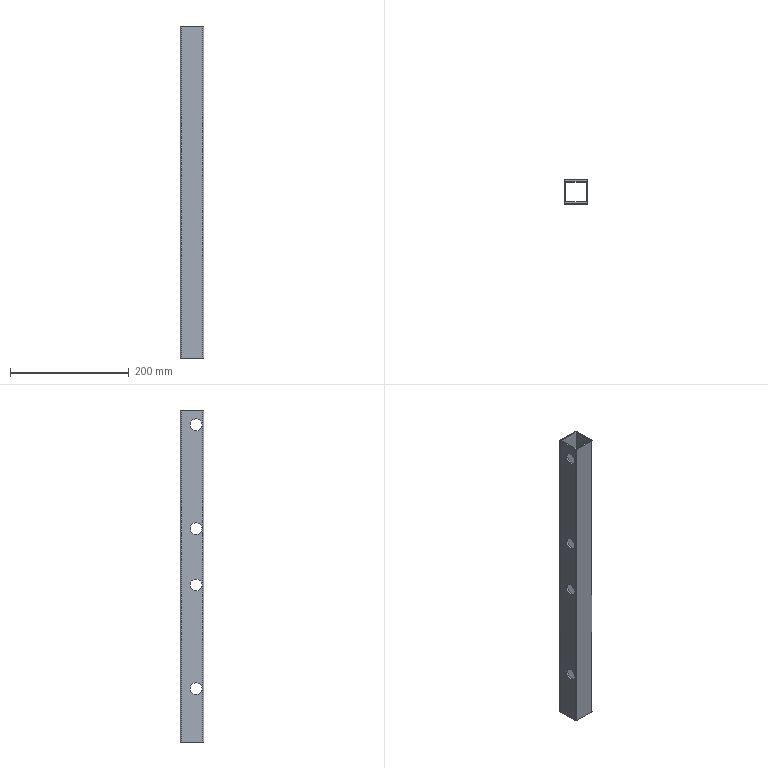Part | STEP file | X77-09107 | 1 solid | 30 faces | box 40 x 40 x 560 mm | volume 239177 mm3 | cylinder 20 | plane 10 | commonest cylinder face diameters 20 x16 4 x4
STEP:
#1=CARTESIAN_POINT('',(0.,3.,90.));
#2=VERTEX_POINT('',#1);
#3=CARTESIAN_POINT('',(0.,23.,90.));
#4=VERTEX_POINT('',#3);
#5=CARTESIAN_POINT('',(0.,13.,90.));
#6=DIRECTION('',(1.,0.,0.));
#7=DIRECTION('',(0.,1.,0.));
#8=AXIS2_PLACEMENT_3D('',#5,#6,#7);
#9=CIRCLE('',#8,10.);
#10=EDGE_CURVE('',#2,#4,#9,.T.);
#11=ORIENTED_EDGE('',*,*,#10,.F.);
#12=CARTESIAN_POINT('',(3.,3.,90.));
#13=VERTEX_POINT('',#12);
#14=CARTESIAN_POINT('',(0.,3.,90.));
#15=DIRECTION('',(1.,0.,0.));
#16=VECTOR('',#15,1000.);
#17=LINE('',#14,#16);
#18=EDGE_CURVE('',#2,#13,#17,.T.);
#19=ORIENTED_EDGE('',*,*,#18,.T.);
#20=CARTESIAN_POINT('',(3.,23.,90.));
#21=VERTEX_POINT('',#20);
#22=CARTESIAN_POINT('',(3.,13.,90.));
#23=DIRECTION('',(1.,0.,0.));
#24=DIRECTION('',(0.,0.,-1.));
#25=AXIS2_PLACEMENT_3D('',#22,#23,#24);
#26=CIRCLE('',#25,10.);
#27=EDGE_CURVE('',#13,#21,#26,.T.);
#28=ORIENTED_EDGE('',*,*,#27,.T.);
#29=CARTESIAN_POINT('',(0.,23.,90.));
#30=DIRECTION('',(1.,0.,0.));
#31=VECTOR('',#30,1000.);
#32=LINE('',#29,#31);
#33=EDGE_CURVE('',#4,#21,#32,.T.);
#34=ORIENTED_EDGE('',*,*,#33,.F.);
#35=EDGE_LOOP('',(#11,#19,#28,#34));
#36=FACE_OUTER_BOUND('',#35,.T.);
#37=CARTESIAN_POINT('',(0.,13.,90.));
#38=DIRECTION('',(1.,0.,0.));
#39=DIRECTION('',(0.,1.,0.));
#40=AXIS2_PLACEMENT_3D('',#37,#38,#39);
#41=CYLINDRICAL_SURFACE('',#40,10.);
#42=ADVANCED_FACE('',(#36),#41,.F.);
#43=CARTESIAN_POINT('',(37.,23.,90.));
#44=VERTEX_POINT('',#43);
#45=CARTESIAN_POINT('',(37.,3.,90.));
#46=VERTEX_POINT('',#45);
#47=CARTESIAN_POINT('',(37.,13.,90.));
#48=DIRECTION('',(-1.,0.,0.));
#49=DIRECTION('',(0.,0.,1.));
#50=AXIS2_PLACEMENT_3D('',#47,#48,#49);
#51=CIRCLE('',#50,10.);
#52=EDGE_CURVE('',#44,#46,#51,.T.);
#53=ORIENTED_EDGE('',*,*,#52,.T.);
#54=CARTESIAN_POINT('',(40.,3.,90.));
#55=VERTEX_POINT('',#54);
#56=CARTESIAN_POINT('',(0.,3.,90.));
#57=DIRECTION('',(1.,0.,0.));
#58=VECTOR('',#57,1000.);
#59=LINE('',#56,#58);
#60=EDGE_CURVE('',#46,#55,#59,.T.);
#61=ORIENTED_EDGE('',*,*,#60,.T.);
#62=CARTESIAN_POINT('',(40.,23.,90.));
#63=VERTEX_POINT('',#62);
#64=CARTESIAN_POINT('',(40.,13.,90.));
#65=DIRECTION('',(1.,0.,0.));
#66=DIRECTION('',(0.,1.,0.));
#67=AXIS2_PLACEMENT_3D('',#64,#65,#66);
#68=CIRCLE('',#67,10.);
#69=EDGE_CURVE('',#55,#63,#68,.T.);
#70=ORIENTED_EDGE('',*,*,#69,.T.);
#71=CARTESIAN_POINT('',(0.,23.,90.));
#72=DIRECTION('',(1.,0.,0.));
#73=VECTOR('',#72,1000.);
#74=LINE('',#71,#73);
#75=EDGE_CURVE('',#44,#63,#74,.T.);
#76=ORIENTED_EDGE('',*,*,#75,.F.);
#77=EDGE_LOOP('',(#53,#61,#70,#76));
#78=FACE_OUTER_BOUND('',#77,.T.);
#79=CARTESIAN_POINT('',(0.,13.,90.));
#80=DIRECTION('',(1.,0.,0.));
#81=DIRECTION('',(0.,1.,0.));
#82=AXIS2_PLACEMENT_3D('',#79,#80,#81);
#83=CYLINDRICAL_SURFACE('',#82,10.);
#84=ADVANCED_FACE('',(#78),#83,.F.);
#85=CARTESIAN_POINT('',(0.,3.,265.));
#86=VERTEX_POINT('',#85);
#87=CARTESIAN_POINT('',(0.,23.,265.));
#88=VERTEX_POINT('',#87);
#89=CARTESIAN_POINT('',(0.,13.,265.));
#90=DIRECTION('',(1.,0.,0.));
#91=DIRECTION('',(0.,1.,0.));
#92=AXIS2_PLACEMENT_3D('',#89,#90,#91);
#93=CIRCLE('',#92,10.);
#94=EDGE_CURVE('',#86,#88,#93,.T.);
#95=ORIENTED_EDGE('',*,*,#94,.F.);
#96=CARTESIAN_POINT('',(3.,3.,265.));
#97=VERTEX_POINT('',#96);
#98=CARTESIAN_POINT('',(0.,3.,265.));
#99=DIRECTION('',(1.,0.,0.));
#100=VECTOR('',#99,1000.);
#101=LINE('',#98,#100);
#102=EDGE_CURVE('',#86,#97,#101,.T.);
#103=ORIENTED_EDGE('',*,*,#102,.T.);
#104=CARTESIAN_POINT('',(3.,23.,265.));
#105=VERTEX_POINT('',#104);
#106=CARTESIAN_POINT('',(3.,13.,265.));
#107=DIRECTION('',(1.,0.,0.));
#108=DIRECTION('',(0.,0.,-1.));
#109=AXIS2_PLACEMENT_3D('',#106,#107,#108);
#110=CIRCLE('',#109,10.);
#111=EDGE_CURVE('',#97,#105,#110,.T.);
#112=ORIENTED_EDGE('',*,*,#111,.T.);
#113=CARTESIAN_POINT('',(0.,23.,265.));
#114=DIRECTION('',(1.,0.,0.));
#115=VECTOR('',#114,1000.);
#116=LINE('',#113,#115);
#117=EDGE_CURVE('',#88,#105,#116,.T.);
#118=ORIENTED_EDGE('',*,*,#117,.F.);
#119=EDGE_LOOP('',(#95,#103,#112,#118));
#120=FACE_OUTER_BOUND('',#119,.T.);
#121=CARTESIAN_POINT('',(0.,13.,265.));
#122=DIRECTION('',(1.,0.,0.));
#123=DIRECTION('',(0.,1.,0.));
#124=AXIS2_PLACEMENT_3D('',#121,#122,#123);
#125=CYLINDRICAL_SURFACE('',#124,10.);
#126=ADVANCED_FACE('',(#120),#125,.F.);
#127=CARTESIAN_POINT('',(37.,23.,265.));
#128=VERTEX_POINT('',#127);
#129=CARTESIAN_POINT('',(37.,3.,265.));
#130=VERTEX_POINT('',#129);
#131=CARTESIAN_POINT('',(37.,13.,265.));
#132=DIRECTION('',(-1.,0.,0.));
#133=DIRECTION('',(0.,0.,1.));
#134=AXIS2_PLACEMENT_3D('',#131,#132,#133);
#135=CIRCLE('',#134,10.);
#136=EDGE_CURVE('',#128,#130,#135,.T.);
#137=ORIENTED_EDGE('',*,*,#136,.T.);
#138=CARTESIAN_POINT('',(40.,3.,265.));
#139=VERTEX_POINT('',#138);
#140=CARTESIAN_POINT('',(0.,3.,265.));
#141=DIRECTION('',(1.,0.,0.));
#142=VECTOR('',#141,1000.);
#143=LINE('',#140,#142);
#144=EDGE_CURVE('',#130,#139,#143,.T.);
#145=ORIENTED_EDGE('',*,*,#144,.T.);
#146=CARTESIAN_POINT('',(40.,23.,265.));
#147=VERTEX_POINT('',#146);
#148=CARTESIAN_POINT('',(40.,13.,265.));
#149=DIRECTION('',(1.,0.,0.));
#150=DIRECTION('',(0.,1.,0.));
#151=AXIS2_PLACEMENT_3D('',#148,#149,#150);
#152=CIRCLE('',#151,10.);
#153=EDGE_CURVE('',#139,#147,#152,.T.);
#154=ORIENTED_EDGE('',*,*,#153,.T.);
#155=CARTESIAN_POINT('',(0.,23.,265.));
#156=DIRECTION('',(1.,0.,0.));
#157=VECTOR('',#156,1000.);
#158=LINE('',#155,#157);
#159=EDGE_CURVE('',#128,#147,#158,.T.);
#160=ORIENTED_EDGE('',*,*,#159,.F.);
#161=EDGE_LOOP('',(#137,#145,#154,#160));
#162=FACE_OUTER_BOUND('',#161,.T.);
#163=CARTESIAN_POINT('',(0.,13.,265.));
#164=DIRECTION('',(1.,0.,0.));
#165=DIRECTION('',(0.,1.,0.));
#166=AXIS2_PLACEMENT_3D('',#163,#164,#165);
#167=CYLINDRICAL_SURFACE('',#166,10.);
#168=ADVANCED_FACE('',(#162),#167,.F.);
#169=CARTESIAN_POINT('',(0.,3.,535.));
#170=VERTEX_POINT('',#169);
#171=CARTESIAN_POINT('',(0.,23.,535.));
#172=VERTEX_POINT('',#171);
#173=CARTESIAN_POINT('',(0.,13.,535.));
#174=DIRECTION('',(1.,0.,0.));
#175=DIRECTION('',(0.,1.,0.));
#176=AXIS2_PLACEMENT_3D('',#173,#174,#175);
#177=CIRCLE('',#176,10.);
#178=EDGE_CURVE('',#170,#172,#177,.T.);
#179=ORIENTED_EDGE('',*,*,#178,.F.);
#180=CARTESIAN_POINT('',(3.,3.,535.));
#181=VERTEX_POINT('',#180);
#182=CARTESIAN_POINT('',(0.,3.,535.));
#183=DIRECTION('',(1.,0.,0.));
#184=VECTOR('',#183,1000.);
#185=LINE('',#182,#184);
#186=EDGE_CURVE('',#170,#181,#185,.T.);
#187=ORIENTED_EDGE('',*,*,#186,.T.);
#188=CARTESIAN_POINT('',(3.,23.,535.));
#189=VERTEX_POINT('',#188);
#190=CARTESIAN_POINT('',(3.,13.,535.));
#191=DIRECTION('',(1.,0.,0.));
#192=DIRECTION('',(0.,0.,-1.));
#193=AXIS2_PLACEMENT_3D('',#190,#191,#192);
#194=CIRCLE('',#193,10.);
#195=EDGE_CURVE('',#181,#189,#194,.T.);
#196=ORIENTED_EDGE('',*,*,#195,.T.);
#197=CARTESIAN_POINT('',(0.,23.,535.));
#198=DIRECTION('',(1.,0.,0.));
#199=VECTOR('',#198,1000.);
#200=LINE('',#197,#199);
#201=EDGE_CURVE('',#172,#189,#200,.T.);
#202=ORIENTED_EDGE('',*,*,#201,.F.);
#203=EDGE_LOOP('',(#179,#187,#196,#202));
#204=FACE_OUTER_BOUND('',#203,.T.);
#205=CARTESIAN_POINT('',(0.,13.,535.));
#206=DIRECTION('',(1.,0.,0.));
#207=DIRECTION('',(0.,1.,0.));
#208=AXIS2_PLACEMENT_3D('',#205,#206,#207);
#209=CYLINDRICAL_SURFACE('',#208,10.);
#210=ADVANCED_FACE('',(#204),#209,.F.);
#211=CARTESIAN_POINT('',(37.,23.,535.));
#212=VERTEX_POINT('',#211);
#213=CARTESIAN_POINT('',(37.,3.,535.));
#214=VERTEX_POINT('',#213);
#215=CARTESIAN_POINT('',(37.,13.,535.));
#216=DIRECTION('',(-1.,0.,0.));
#217=DIRECTION('',(0.,0.,1.));
#218=AXIS2_PLACEMENT_3D('',#215,#216,#217);
#219=CIRCLE('',#218,10.);
#220=EDGE_CURVE('',#212,#214,#219,.T.);
#221=ORIENTED_EDGE('',*,*,#220,.T.);
#222=CARTESIAN_POINT('',(40.,3.,535.));
#223=VERTEX_POINT('',#222);
#224=CARTESIAN_POINT('',(0.,3.,535.));
#225=DIRECTION('',(1.,0.,0.));
#226=VECTOR('',#225,1000.);
#227=LINE('',#224,#226);
#228=EDGE_CURVE('',#214,#223,#227,.T.);
#229=ORIENTED_EDGE('',*,*,#228,.T.);
#230=CARTESIAN_POINT('',(40.,23.,535.));
#231=VERTEX_POINT('',#230);
#232=CARTESIAN_POINT('',(40.,13.,535.));
#233=DIRECTION('',(1.,0.,0.));
#234=DIRECTION('',(0.,1.,0.));
#235=AXIS2_PLACEMENT_3D('',#232,#233,#234);
#236=CIRCLE('',#235,10.);
#237=EDGE_CURVE('',#223,#231,#236,.T.);
#238=ORIENTED_EDGE('',*,*,#237,.T.);
#239=CARTESIAN_POINT('',(0.,23.,535.));
#240=DIRECTION('',(1.,0.,0.));
#241=VECTOR('',#240,1000.);
#242=LINE('',#239,#241);
#243=EDGE_CURVE('',#212,#231,#242,.T.);
#244=ORIENTED_EDGE('',*,*,#243,.F.);
#245=EDGE_LOOP('',(#221,#229,#238,#244));
#246=FACE_OUTER_BOUND('',#245,.T.);
#247=CARTESIAN_POINT('',(0.,13.,535.));
#248=DIRECTION('',(1.,0.,0.));
#249=DIRECTION('',(0.,1.,0.));
#250=AXIS2_PLACEMENT_3D('',#247,#248,#249);
#251=CYLINDRICAL_SURFACE('',#250,10.);
#252=ADVANCED_FACE('',(#246),#251,.F.);
#253=CARTESIAN_POINT('',(0.,3.,360.));
#254=VERTEX_POINT('',#253);
#255=CARTESIAN_POINT('',(0.,23.,360.));
#256=VERTEX_POINT('',#255);
#257=CARTESIAN_POINT('',(0.,13.,360.));
#258=DIRECTION('',(1.,0.,0.));
#259=DIRECTION('',(0.,1.,0.));
#260=AXIS2_PLACEMENT_3D('',#257,#258,#259);
#261=CIRCLE('',#260,10.);
#262=EDGE_CURVE('',#254,#256,#261,.T.);
#263=ORIENTED_EDGE('',*,*,#262,.F.);
#264=CARTESIAN_POINT('',(3.,3.,360.));
#265=VERTEX_POINT('',#264);
#266=CARTESIAN_POINT('',(0.,3.,360.));
#267=DIRECTION('',(1.,0.,0.));
#268=VECTOR('',#267,1000.);
#269=LINE('',#266,#268);
#270=EDGE_CURVE('',#254,#265,#269,.T.);
#271=ORIENTED_EDGE('',*,*,#270,.T.);
#272=CARTESIAN_POINT('',(3.,23.,360.));
#273=VERTEX_POINT('',#272);
#274=CARTESIAN_POINT('',(3.,13.,360.));
#275=DIRECTION('',(1.,0.,0.));
#276=DIRECTION('',(0.,0.,-1.));
#277=AXIS2_PLACEMENT_3D('',#274,#275,#276);
#278=CIRCLE('',#277,10.);
#279=EDGE_CURVE('',#265,#273,#278,.T.);
#280=ORIENTED_EDGE('',*,*,#279,.T.);
#281=CARTESIAN_POINT('',(0.,23.,360.));
#282=DIRECTION('',(1.,0.,0.));
#283=VECTOR('',#282,1000.);
#284=LINE('',#281,#283);
#285=EDGE_CURVE('',#256,#273,#284,.T.);
#286=ORIENTED_EDGE('',*,*,#285,.F.);
#287=EDGE_LOOP('',(#263,#271,#280,#286));
#288=FACE_OUTER_BOUND('',#287,.T.);
#289=CARTESIAN_POINT('',(0.,13.,360.));
#290=DIRECTION('',(1.,0.,0.));
#291=DIRECTION('',(0.,1.,0.));
#292=AXIS2_PLACEMENT_3D('',#289,#290,#291);
#293=CYLINDRICAL_SURFACE('',#292,10.);
#294=ADVANCED_FACE('',(#288),#293,.F.);
#295=CARTESIAN_POINT('',(37.,23.,360.));
#296=VERTEX_POINT('',#295);
#297=CARTESIAN_POINT('',(37.,3.,360.));
#298=VERTEX_POINT('',#297);
#299=CARTESIAN_POINT('',(37.,13.,360.));
#300=DIRECTION('',(-1.,0.,0.));
#301=DIRECTION('',(0.,0.,1.));
#302=AXIS2_PLACEMENT_3D('',#299,#300,#301);
#303=CIRCLE('',#302,10.);
#304=EDGE_CURVE('',#296,#298,#303,.T.);
#305=ORIENTED_EDGE('',*,*,#304,.T.);
#306=CARTESIAN_POINT('',(40.,3.,360.));
#307=VERTEX_POINT('',#306);
#308=CARTESIAN_POINT('',(0.,3.,360.));
#309=DIRECTION('',(1.,0.,0.));
#310=VECTOR('',#309,1000.);
#311=LINE('',#308,#310);
#312=EDGE_CURVE('',#298,#307,#311,.T.);
#313=ORIENTED_EDGE('',*,*,#312,.T.);
#314=CARTESIAN_POINT('',(40.,23.,360.));
#315=VERTEX_POINT('',#314);
#316=CARTESIAN_POINT('',(40.,13.,360.));
#317=DIRECTION('',(1.,0.,0.));
#318=DIRECTION('',(0.,1.,0.));
#319=AXIS2_PLACEMENT_3D('',#316,#317,#318);
#320=CIRCLE('',#319,10.);
#321=EDGE_CURVE('',#307,#315,#320,.T.);
#322=ORIENTED_EDGE('',*,*,#321,.T.);
#323=CARTESIAN_POINT('',(0.,23.,360.));
#324=DIRECTION('',(1.,0.,0.));
#325=VECTOR('',#324,1000.);
#326=LINE('',#323,#325);
#327=EDGE_CURVE('',#296,#315,#326,.T.);
#328=ORIENTED_EDGE('',*,*,#327,.F.);
#329=EDGE_LOOP('',(#305,#313,#322,#328));
#330=FACE_OUTER_BOUND('',#329,.T.);
#331=CARTESIAN_POINT('',(0.,13.,360.));
#332=DIRECTION('',(1.,0.,0.));
#333=DIRECTION('',(0.,1.,0.));
#334=AXIS2_PLACEMENT_3D('',#331,#332,#333);
#335=CYLINDRICAL_SURFACE('',#334,10.);
#336=ADVANCED_FACE('',(#330),#335,.F.);
#337=CARTESIAN_POINT('',(0.,2.,560.));
#338=VERTEX_POINT('',#337);
#339=CARTESIAN_POINT('',(2.,0.,560.));
#340=VERTEX_POINT('',#339);
#341=CARTESIAN_POINT('',(2.,2.,560.));
#342=DIRECTION('',(0.,0.,1.));
#343=DIRECTION('',(1.,0.,0.));
#344=AXIS2_PLACEMENT_3D('',#341,#342,#343);
#345=CIRCLE('',#344,2.);
#346=EDGE_CURVE('',#338,#340,#345,.T.);
#347=ORIENTED_EDGE('',*,*,#346,.T.);
#348=CARTESIAN_POINT('',(38.,0.,560.));
#349=VERTEX_POINT('',#348);
#350=CARTESIAN_POINT('',(2.,0.,560.));
#351=DIRECTION('',(1.,0.,0.));
#352=VECTOR('',#351,1000.);
#353=LINE('',#350,#352);
#354=EDGE_CURVE('',#340,#349,#353,.T.);
#355=ORIENTED_EDGE('',*,*,#354,.T.);
#356=CARTESIAN_POINT('',(40.,2.,560.));
#357=VERTEX_POINT('',#356);
#358=CARTESIAN_POINT('',(38.,2.,560.));
#359=DIRECTION('',(0.,0.,1.));
#360=DIRECTION('',(1.,0.,0.));
#361=AXIS2_PLACEMENT_3D('',#358,#359,#360);
#362=CIRCLE('',#361,2.);
#363=EDGE_CURVE('',#349,#357,#362,.T.);
#364=ORIENTED_EDGE('',*,*,#363,.T.);
#365=CARTESIAN_POINT('',(40.,38.,560.));
#366=VERTEX_POINT('',#365);
#367=CARTESIAN_POINT('',(40.,2.,560.));
#368=DIRECTION('',(0.,1.,0.));
#369=VECTOR('',#368,1000.);
#370=LINE('',#367,#369);
#371=EDGE_CURVE('',#357,#366,#370,.T.);
#372=ORIENTED_EDGE('',*,*,#371,.T.);
#373=CARTESIAN_POINT('',(38.,40.,560.));
#374=VERTEX_POINT('',#373);
#375=CARTESIAN_POINT('',(38.,38.,560.));
#376=DIRECTION('',(0.,0.,1.));
#377=DIRECTION('',(1.,0.,0.));
#378=AXIS2_PLACEMENT_3D('',#375,#376,#377);
#379=CIRCLE('',#378,2.);
#380=EDGE_CURVE('',#366,#374,#379,.T.);
#381=ORIENTED_EDGE('',*,*,#380,.T.);
#382=CARTESIAN_POINT('',(2.,40.,560.));
#383=VERTEX_POINT('',#382);
#384=CARTESIAN_POINT('',(2.,40.,560.));
#385=DIRECTION('',(-1.,0.,0.));
#386=VECTOR('',#385,1000.);
#387=LINE('',#384,#386);
#388=EDGE_CURVE('',#374,#383,#387,.T.);
#389=ORIENTED_EDGE('',*,*,#388,.T.);
#390=CARTESIAN_POINT('',(0.,38.,560.));
#391=VERTEX_POINT('',#390);
#392=CARTESIAN_POINT('',(2.,38.,560.));
#393=DIRECTION('',(0.,0.,1.));
#394=DIRECTION('',(-1.,0.,0.));
#395=AXIS2_PLACEMENT_3D('',#392,#393,#394);
#396=CIRCLE('',#395,2.);
#397=EDGE_CURVE('',#383,#391,#396,.T.);
#398=ORIENTED_EDGE('',*,*,#397,.T.);
#399=CARTESIAN_POINT('',(0.,2.,560.));
#400=DIRECTION('',(0.,-1.,0.));
#401=VECTOR('',#400,1000.);
#402=LINE('',#399,#401);
#403=EDGE_CURVE('',#391,#338,#402,.T.);
#404=ORIENTED_EDGE('',*,*,#403,.T.);
#405=EDGE_LOOP('',(#347,#355,#364,#372,#381,#389,#398,#404));
#406=FACE_OUTER_BOUND('',#405,.T.);
#407=CARTESIAN_POINT('',(3.,3.,560.));
#408=VERTEX_POINT('',#407);
#409=CARTESIAN_POINT('',(37.,3.,560.));
#410=VERTEX_POINT('',#409);
#411=CARTESIAN_POINT('',(3.,3.,560.));
#412=DIRECTION('',(1.,0.,0.));
#413=VECTOR('',#412,1000.);
#414=LINE('',#411,#413);
#415=EDGE_CURVE('',#408,#410,#414,.T.);
#416=ORIENTED_EDGE('',*,*,#415,.F.);
#417=CARTESIAN_POINT('',(3.,37.,560.));
#418=VERTEX_POINT('',#417);
#419=CARTESIAN_POINT('',(3.,3.,560.));
#420=DIRECTION('',(0.,-1.,0.));
#421=VECTOR('',#420,1000.);
#422=LINE('',#419,#421);
#423=EDGE_CURVE('',#418,#408,#422,.T.);
#424=ORIENTED_EDGE('',*,*,#423,.F.);
#425=CARTESIAN_POINT('',(37.,37.,560.));
#426=VERTEX_POINT('',#425);
#427=CARTESIAN_POINT('',(3.,37.,560.));
#428=DIRECTION('',(-1.,0.,0.));
#429=VECTOR('',#428,1000.);
#430=LINE('',#427,#429);
#431=EDGE_CURVE('',#426,#418,#430,.T.);
#432=ORIENTED_EDGE('',*,*,#431,.F.);
#433=CARTESIAN_POINT('',(37.,3.,560.));
#434=DIRECTION('',(0.,1.,0.));
#435=VECTOR('',#434,1000.);
#436=LINE('',#433,#435);
#437=EDGE_CURVE('',#410,#426,#436,.T.);
#438=ORIENTED_EDGE('',*,*,#437,.F.);
#439=EDGE_LOOP('',(#416,#424,#432,#438));
#440=FACE_BOUND('',#439,.T.);
#441=CARTESIAN_POINT('',(2.,2.,560.));
#442=DIRECTION('',(0.,0.,1.));
#443=DIRECTION('',(1.,0.,0.));
#444=AXIS2_PLACEMENT_3D('',#441,#442,#443);
#445=PLANE('',#444);
#446=ADVANCED_FACE('',(#406,#440),#445,.T.);
#447=CARTESIAN_POINT('',(0.,2.,0.));
#448=VERTEX_POINT('',#447);
#449=CARTESIAN_POINT('',(2.,0.,0.));
#450=VERTEX_POINT('',#449);
#451=CARTESIAN_POINT('',(2.,2.,0.));
#452=DIRECTION('',(0.,0.,1.));
#453=DIRECTION('',(1.,0.,0.));
#454=AXIS2_PLACEMENT_3D('',#451,#452,#453);
#455=CIRCLE('',#454,2.);
#456=EDGE_CURVE('',#448,#450,#455,.T.);
#457=ORIENTED_EDGE('',*,*,#456,.F.);
#458=CARTESIAN_POINT('',(0.,38.,0.));
#459=VERTEX_POINT('',#458);
#460=CARTESIAN_POINT('',(0.,2.,0.));
#461=DIRECTION('',(0.,-1.,0.));
#462=VECTOR('',#461,1000.);
#463=LINE('',#460,#462);
#464=EDGE_CURVE('',#459,#448,#463,.T.);
#465=ORIENTED_EDGE('',*,*,#464,.F.);
#466=CARTESIAN_POINT('',(2.,40.,0.));
#467=VERTEX_POINT('',#466);
#468=CARTESIAN_POINT('',(2.,38.,0.));
#469=DIRECTION('',(0.,0.,1.));
#470=DIRECTION('',(-1.,0.,0.));
#471=AXIS2_PLACEMENT_3D('',#468,#469,#470);
#472=CIRCLE('',#471,2.);
#473=EDGE_CURVE('',#467,#459,#472,.T.);
#474=ORIENTED_EDGE('',*,*,#473,.F.);
#475=CARTESIAN_POINT('',(38.,40.,0.));
#476=VERTEX_POINT('',#475);
#477=CARTESIAN_POINT('',(2.,40.,0.));
#478=DIRECTION('',(-1.,0.,0.));
#479=VECTOR('',#478,1000.);
#480=LINE('',#477,#479);
#481=EDGE_CURVE('',#476,#467,#480,.T.);
#482=ORIENTED_EDGE('',*,*,#481,.F.);
#483=CARTESIAN_POINT('',(40.,38.,0.));
#484=VERTEX_POINT('',#483);
#485=CARTESIAN_POINT('',(38.,38.,0.));
#486=DIRECTION('',(0.,0.,1.));
#487=DIRECTION('',(1.,0.,0.));
#488=AXIS2_PLACEMENT_3D('',#485,#486,#487);
#489=CIRCLE('',#488,2.);
#490=EDGE_CURVE('',#484,#476,#489,.T.);
#491=ORIENTED_EDGE('',*,*,#490,.F.);
#492=CARTESIAN_POINT('',(40.,2.,0.));
#493=VERTEX_POINT('',#492);
#494=CARTESIAN_POINT('',(40.,2.,0.));
#495=DIRECTION('',(0.,1.,0.));
#496=VECTOR('',#495,1000.);
#497=LINE('',#494,#496);
#498=EDGE_CURVE('',#493,#484,#497,.T.);
#499=ORIENTED_EDGE('',*,*,#498,.F.);
#500=CARTESIAN_POINT('',(38.,0.,0.));
#501=VERTEX_POINT('',#500);
#502=CARTESIAN_POINT('',(38.,2.,0.));
#503=DIRECTION('',(0.,0.,1.));
#504=DIRECTION('',(1.,0.,0.));
#505=AXIS2_PLACEMENT_3D('',#502,#503,#504);
#506=CIRCLE('',#505,2.);
#507=EDGE_CURVE('',#501,#493,#506,.T.);
#508=ORIENTED_EDGE('',*,*,#507,.F.);
#509=CARTESIAN_POINT('',(2.,0.,0.));
#510=DIRECTION('',(1.,0.,0.));
#511=VECTOR('',#510,1000.);
#512=LINE('',#509,#511);
#513=EDGE_CURVE('',#450,#501,#512,.T.);
#514=ORIENTED_EDGE('',*,*,#513,.F.);
#515=EDGE_LOOP('',(#457,#465,#474,#482,#491,#499,#508,#514));
#516=FACE_OUTER_BOUND('',#515,.T.);
#517=CARTESIAN_POINT('',(3.,37.,0.));
#518=VERTEX_POINT('',#517);
#519=CARTESIAN_POINT('',(3.,3.,0.));
#520=VERTEX_POINT('',#519);
#521=CARTESIAN_POINT('',(3.,3.,0.));
#522=DIRECTION('',(0.,-1.,0.));
#523=VECTOR('',#522,1000.);
#524=LINE('',#521,#523);
#525=EDGE_CURVE('',#518,#520,#524,.T.);
#526=ORIENTED_EDGE('',*,*,#525,.T.);
#527=CARTESIAN_POINT('',(37.,3.,0.));
#528=VERTEX_POINT('',#527);
#529=CARTESIAN_POINT('',(3.,3.,0.));
#530=DIRECTION('',(1.,0.,0.));
#531=VECTOR('',#530,1000.);
#532=LINE('',#529,#531);
#533=EDGE_CURVE('',#520,#528,#532,.T.);
#534=ORIENTED_EDGE('',*,*,#533,.T.);
#535=CARTESIAN_POINT('',(37.,37.,0.));
#536=VERTEX_POINT('',#535);
#537=CARTESIAN_POINT('',(37.,3.,0.));
#538=DIRECTION('',(0.,1.,0.));
#539=VECTOR('',#538,1000.);
#540=LINE('',#537,#539);
#541=EDGE_CURVE('',#528,#536,#540,.T.);
#542=ORIENTED_EDGE('',*,*,#541,.T.);
#543=CARTESIAN_POINT('',(3.,37.,0.));
#544=DIRECTION('',(-1.,0.,0.));
#545=VECTOR('',#544,1000.);
#546=LINE('',#543,#545);
#547=EDGE_CURVE('',#536,#518,#546,.T.);
#548=ORIENTED_EDGE('',*,*,#547,.T.);
#549=EDGE_LOOP('',(#526,#534,#542,#548));
#550=FACE_BOUND('',#549,.T.);
#551=CARTESIAN_POINT('',(2.,2.,0.));
#552=DIRECTION('',(0.,0.,1.));
#553=DIRECTION('',(1.,0.,0.));
#554=AXIS2_PLACEMENT_3D('',#551,#552,#553);
#555=PLANE('',#554);
#556=ADVANCED_FACE('',(#516,#550),#555,.F.);
#557=ORIENTED_EDGE('',*,*,#456,.T.);
#558=CARTESIAN_POINT('',(2.,0.,560.));
#559=DIRECTION('',(0.,0.,-1.));
#560=VECTOR('',#559,1000.);
#561=LINE('',#558,#560);
#562=EDGE_CURVE('',#340,#450,#561,.T.);
#563=ORIENTED_EDGE('',*,*,#562,.F.);
#564=ORIENTED_EDGE('',*,*,#346,.F.);
#565=CARTESIAN_POINT('',(0.,2.,560.));
#566=DIRECTION('',(0.,0.,-1.));
#567=VECTOR('',#566,1000.);
#568=LINE('',#565,#567);
#569=EDGE_CURVE('',#338,#448,#568,.T.);
#570=ORIENTED_EDGE('',*,*,#569,.T.);
#571=EDGE_LOOP('',(#557,#563,#564,#570));
#572=FACE_OUTER_BOUND('',#571,.T.);
#573=CARTESIAN_POINT('',(2.,2.,560.));
#574=DIRECTION('',(0.,0.,-1.));
#575=DIRECTION('',(-1.,0.,0.));
#576=AXIS2_PLACEMENT_3D('',#573,#574,#575);
#577=CYLINDRICAL_SURFACE('',#576,2.);
#578=ADVANCED_FACE('',(#572),#577,.T.);
#579=ORIENTED_EDGE('',*,*,#513,.T.);
#580=CARTESIAN_POINT('',(38.,0.,560.));
#581=DIRECTION('',(0.,0.,-1.));
#582=VECTOR('',#581,1000.);
#583=LINE('',#580,#582);
#584=EDGE_CURVE('',#349,#501,#583,.T.);
#585=ORIENTED_EDGE('',*,*,#584,.F.);
#586=ORIENTED_EDGE('',*,*,#354,.F.);
#587=ORIENTED_EDGE('',*,*,#562,.T.);
#588=EDGE_LOOP('',(#579,#585,#586,#587));
#589=FACE_OUTER_BOUND('',#588,.T.);
#590=CARTESIAN_POINT('',(2.,0.,560.));
#591=DIRECTION('',(0.,1.,0.));
#592=DIRECTION('',(0.,0.,1.));
#593=AXIS2_PLACEMENT_3D('',#590,#591,#592);
#594=PLANE('',#593);
#595=ADVANCED_FACE('',(#589),#594,.F.);
#596=ORIENTED_EDGE('',*,*,#507,.T.);
#597=CARTESIAN_POINT('',(40.,2.,560.));
#598=DIRECTION('',(0.,0.,-1.));
#599=VECTOR('',#598,1000.);
#600=LINE('',#597,#599);
#601=EDGE_CURVE('',#357,#493,#600,.T.);
#602=ORIENTED_EDGE('',*,*,#601,.F.);
#603=ORIENTED_EDGE('',*,*,#363,.F.);
#604=ORIENTED_EDGE('',*,*,#584,.T.);
#605=EDGE_LOOP('',(#596,#602,#603,#604));
#606=FACE_OUTER_BOUND('',#605,.T.);
#607=CARTESIAN_POINT('',(38.,2.,560.));
#608=DIRECTION('',(0.,0.,-1.));
#609=DIRECTION('',(-1.,0.,0.));
#610=AXIS2_PLACEMENT_3D('',#607,#608,#609);
#611=CYLINDRICAL_SURFACE('',#610,2.);
#612=ADVANCED_FACE('',(#606),#611,.T.);
#613=CARTESIAN_POINT('',(40.,13.,90.));
#614=DIRECTION('',(1.,0.,0.));
#615=DIRECTION('',(0.,1.,0.));
#616=AXIS2_PLACEMENT_3D('',#613,#614,#615);
#617=CIRCLE('',#616,10.);
#618=EDGE_CURVE('',#63,#55,#617,.T.);
#619=ORIENTED_EDGE('',*,*,#618,.F.);
#620=ORIENTED_EDGE('',*,*,#69,.F.);
#621=EDGE_LOOP('',(#619,#620));
#622=FACE_BOUND('',#621,.T.);
#623=CARTESIAN_POINT('',(40.,13.,265.));
#624=DIRECTION('',(1.,0.,0.));
#625=DIRECTION('',(0.,1.,0.));
#626=AXIS2_PLACEMENT_3D('',#623,#624,#625);
#627=CIRCLE('',#626,10.);
#628=EDGE_CURVE('',#147,#139,#627,.T.);
#629=ORIENTED_EDGE('',*,*,#628,.F.);
#630=ORIENTED_EDGE('',*,*,#153,.F.);
#631=EDGE_LOOP('',(#629,#630));
#632=FACE_BOUND('',#631,.T.);
#633=CARTESIAN_POINT('',(40.,13.,535.));
#634=DIRECTION('',(1.,0.,0.));
#635=DIRECTION('',(0.,1.,0.));
#636=AXIS2_PLACEMENT_3D('',#633,#634,#635);
#637=CIRCLE('',#636,10.);
#638=EDGE_CURVE('',#231,#223,#637,.T.);
#639=ORIENTED_EDGE('',*,*,#638,.F.);
#640=ORIENTED_EDGE('',*,*,#237,.F.);
#641=EDGE_LOOP('',(#639,#640));
#642=FACE_BOUND('',#641,.T.);
#643=CARTESIAN_POINT('',(40.,13.,360.));
#644=DIRECTION('',(1.,0.,0.));
#645=DIRECTION('',(0.,1.,0.));
#646=AXIS2_PLACEMENT_3D('',#643,#644,#645);
#647=CIRCLE('',#646,10.);
#648=EDGE_CURVE('',#315,#307,#647,.T.);
#649=ORIENTED_EDGE('',*,*,#648,.F.);
#650=ORIENTED_EDGE('',*,*,#321,.F.);
#651=EDGE_LOOP('',(#649,#650));
#652=FACE_BOUND('',#651,.T.);
#653=ORIENTED_EDGE('',*,*,#498,.T.);
#654=CARTESIAN_POINT('',(40.,38.,560.));
#655=DIRECTION('',(0.,0.,-1.));
#656=VECTOR('',#655,1000.);
#657=LINE('',#654,#656);
#658=EDGE_CURVE('',#366,#484,#657,.T.);
#659=ORIENTED_EDGE('',*,*,#658,.F.);
#660=ORIENTED_EDGE('',*,*,#371,.F.);
#661=ORIENTED_EDGE('',*,*,#601,.T.);
#662=EDGE_LOOP('',(#653,#659,#660,#661));
#663=FACE_OUTER_BOUND('',#662,.T.);
#664=CARTESIAN_POINT('',(40.,2.,560.));
#665=DIRECTION('',(-1.,0.,0.));
#666=DIRECTION('',(0.,-1.,0.));
#667=AXIS2_PLACEMENT_3D('',#664,#665,#666);
#668=PLANE('',#667);
#669=ADVANCED_FACE('',(#622,#632,#642,#652,#663),#668,.F.);
#670=ORIENTED_EDGE('',*,*,#490,.T.);
#671=CARTESIAN_POINT('',(38.,40.,560.));
#672=DIRECTION('',(0.,0.,-1.));
#673=VECTOR('',#672,1000.);
#674=LINE('',#671,#673);
#675=EDGE_CURVE('',#374,#476,#674,.T.);
#676=ORIENTED_EDGE('',*,*,#675,.F.);
#677=ORIENTED_EDGE('',*,*,#380,.F.);
#678=ORIENTED_EDGE('',*,*,#658,.T.);
#679=EDGE_LOOP('',(#670,#676,#677,#678));
#680=FACE_OUTER_BOUND('',#679,.T.);
#681=CARTESIAN_POINT('',(38.,38.,560.));
#682=DIRECTION('',(0.,0.,-1.));
#683=DIRECTION('',(-1.,0.,0.));
#684=AXIS2_PLACEMENT_3D('',#681,#682,#683);
#685=CYLINDRICAL_SURFACE('',#684,2.);
#686=ADVANCED_FACE('',(#680),#685,.T.);
#687=ORIENTED_EDGE('',*,*,#481,.T.);
#688=CARTESIAN_POINT('',(2.,40.,560.));
#689=DIRECTION('',(0.,0.,-1.));
#690=VECTOR('',#689,1000.);
#691=LINE('',#688,#690);
#692=EDGE_CURVE('',#383,#467,#691,.T.);
#693=ORIENTED_EDGE('',*,*,#692,.F.);
#694=ORIENTED_EDGE('',*,*,#388,.F.);
#695=ORIENTED_EDGE('',*,*,#675,.T.);
#696=EDGE_LOOP('',(#687,#693,#694,#695));
#697=FACE_OUTER_BOUND('',#696,.T.);
#698=CARTESIAN_POINT('',(2.,40.,560.));
#699=DIRECTION('',(0.,-1.,0.));
#700=DIRECTION('',(0.,0.,-1.));
#701=AXIS2_PLACEMENT_3D('',#698,#699,#700);
#702=PLANE('',#701);
#703=ADVANCED_FACE('',(#697),#702,.F.);
#704=ORIENTED_EDGE('',*,*,#473,.T.);
#705=CARTESIAN_POINT('',(0.,38.,560.));
#706=DIRECTION('',(0.,0.,-1.));
#707=VECTOR('',#706,1000.);
#708=LINE('',#705,#707);
#709=EDGE_CURVE('',#391,#459,#708,.T.);
#710=ORIENTED_EDGE('',*,*,#709,.F.);
#711=ORIENTED_EDGE('',*,*,#397,.F.);
#712=ORIENTED_EDGE('',*,*,#692,.T.);
#713=EDGE_LOOP('',(#704,#710,#711,#712));
#714=FACE_OUTER_BOUND('',#713,.T.);
#715=CARTESIAN_POINT('',(2.,38.,560.));
#716=DIRECTION('',(0.,0.,-1.));
#717=DIRECTION('',(-1.,0.,0.));
#718=AXIS2_PLACEMENT_3D('',#715,#716,#717);
#719=CYLINDRICAL_SURFACE('',#718,2.);
#720=ADVANCED_FACE('',(#714),#719,.T.);
#721=CARTESIAN_POINT('',(0.,13.,90.));
#722=DIRECTION('',(1.,0.,0.));
#723=DIRECTION('',(0.,1.,0.));
#724=AXIS2_PLACEMENT_3D('',#721,#722,#723);
#725=CIRCLE('',#724,10.);
#726=EDGE_CURVE('',#4,#2,#725,.T.);
#727=ORIENTED_EDGE('',*,*,#726,.T.);
#728=ORIENTED_EDGE('',*,*,#10,.T.);
#729=EDGE_LOOP('',(#727,#728));
#730=FACE_BOUND('',#729,.T.);
#731=CARTESIAN_POINT('',(0.,13.,265.));
#732=DIRECTION('',(1.,0.,0.));
#733=DIRECTION('',(0.,1.,0.));
#734=AXIS2_PLACEMENT_3D('',#731,#732,#733);
#735=CIRCLE('',#734,10.);
#736=EDGE_CURVE('',#88,#86,#735,.T.);
#737=ORIENTED_EDGE('',*,*,#736,.T.);
#738=ORIENTED_EDGE('',*,*,#94,.T.);
#739=EDGE_LOOP('',(#737,#738));
#740=FACE_BOUND('',#739,.T.);
#741=CARTESIAN_POINT('',(0.,13.,535.));
#742=DIRECTION('',(1.,0.,0.));
#743=DIRECTION('',(0.,1.,0.));
#744=AXIS2_PLACEMENT_3D('',#741,#742,#743);
#745=CIRCLE('',#744,10.);
#746=EDGE_CURVE('',#172,#170,#745,.T.);
#747=ORIENTED_EDGE('',*,*,#746,.T.);
#748=ORIENTED_EDGE('',*,*,#178,.T.);
#749=EDGE_LOOP('',(#747,#748));
#750=FACE_BOUND('',#749,.T.);
#751=CARTESIAN_POINT('',(0.,13.,360.));
#752=DIRECTION('',(1.,0.,0.));
#753=DIRECTION('',(0.,1.,0.));
#754=AXIS2_PLACEMENT_3D('',#751,#752,#753);
#755=CIRCLE('',#754,10.);
#756=EDGE_CURVE('',#256,#254,#755,.T.);
#757=ORIENTED_EDGE('',*,*,#756,.T.);
#758=ORIENTED_EDGE('',*,*,#262,.T.);
#759=EDGE_LOOP('',(#757,#758));
#760=FACE_BOUND('',#759,.T.);
#761=ORIENTED_EDGE('',*,*,#464,.T.);
#762=ORIENTED_EDGE('',*,*,#569,.F.);
#763=ORIENTED_EDGE('',*,*,#403,.F.);
#764=ORIENTED_EDGE('',*,*,#709,.T.);
#765=EDGE_LOOP('',(#761,#762,#763,#764));
#766=FACE_OUTER_BOUND('',#765,.T.);
#767=CARTESIAN_POINT('',(0.,2.,560.));
#768=DIRECTION('',(1.,0.,0.));
#769=DIRECTION('',(0.,1.,0.));
#770=AXIS2_PLACEMENT_3D('',#767,#768,#769);
#771=PLANE('',#770);
#772=ADVANCED_FACE('',(#730,#740,#750,#760,#766),#771,.F.);
#773=CARTESIAN_POINT('',(3.,3.,560.));
#774=DIRECTION('',(0.,0.,-1.));
#775=VECTOR('',#774,1000.);
#776=LINE('',#773,#775);
#777=EDGE_CURVE('',#97,#13,#776,.T.);
#778=ORIENTED_EDGE('',*,*,#777,.T.);
#779=CARTESIAN_POINT('',(3.,13.,90.));
#780=DIRECTION('',(1.,0.,0.));
#781=DIRECTION('',(0.,0.,-1.));
#782=AXIS2_PLACEMENT_3D('',#779,#780,#781);
#783=CIRCLE('',#782,10.);
#784=EDGE_CURVE('',#21,#13,#783,.T.);
#785=ORIENTED_EDGE('',*,*,#784,.F.);
#786=ORIENTED_EDGE('',*,*,#27,.F.);
#787=CARTESIAN_POINT('',(3.,3.,560.));
#788=DIRECTION('',(0.,0.,-1.));
#789=VECTOR('',#788,1000.);
#790=LINE('',#787,#789);
#791=EDGE_CURVE('',#13,#520,#790,.T.);
#792=ORIENTED_EDGE('',*,*,#791,.T.);
#793=ORIENTED_EDGE('',*,*,#525,.F.);
#794=CARTESIAN_POINT('',(3.,37.,560.));
#795=DIRECTION('',(0.,0.,-1.));
#796=VECTOR('',#795,1000.);
#797=LINE('',#794,#796);
#798=EDGE_CURVE('',#418,#518,#797,.T.);
#799=ORIENTED_EDGE('',*,*,#798,.F.);
#800=ORIENTED_EDGE('',*,*,#423,.T.);
#801=CARTESIAN_POINT('',(3.,3.,560.));
#802=DIRECTION('',(0.,0.,-1.));
#803=VECTOR('',#802,1000.);
#804=LINE('',#801,#803);
#805=EDGE_CURVE('',#408,#181,#804,.T.);
#806=ORIENTED_EDGE('',*,*,#805,.T.);
#807=CARTESIAN_POINT('',(3.,13.,535.));
#808=DIRECTION('',(1.,0.,0.));
#809=DIRECTION('',(0.,0.,-1.));
#810=AXIS2_PLACEMENT_3D('',#807,#808,#809);
#811=CIRCLE('',#810,10.);
#812=EDGE_CURVE('',#189,#181,#811,.T.);
#813=ORIENTED_EDGE('',*,*,#812,.F.);
#814=ORIENTED_EDGE('',*,*,#195,.F.);
#815=CARTESIAN_POINT('',(3.,3.,560.));
#816=DIRECTION('',(0.,0.,-1.));
#817=VECTOR('',#816,1000.);
#818=LINE('',#815,#817);
#819=EDGE_CURVE('',#181,#265,#818,.T.);
#820=ORIENTED_EDGE('',*,*,#819,.T.);
#821=CARTESIAN_POINT('',(3.,13.,360.));
#822=DIRECTION('',(1.,0.,0.));
#823=DIRECTION('',(0.,0.,-1.));
#824=AXIS2_PLACEMENT_3D('',#821,#822,#823);
#825=CIRCLE('',#824,10.);
#826=EDGE_CURVE('',#273,#265,#825,.T.);
#827=ORIENTED_EDGE('',*,*,#826,.F.);
#828=ORIENTED_EDGE('',*,*,#279,.F.);
#829=CARTESIAN_POINT('',(3.,3.,560.));
#830=DIRECTION('',(0.,0.,-1.));
#831=VECTOR('',#830,1000.);
#832=LINE('',#829,#831);
#833=EDGE_CURVE('',#265,#97,#832,.T.);
#834=ORIENTED_EDGE('',*,*,#833,.T.);
#835=CARTESIAN_POINT('',(3.,13.,265.));
#836=DIRECTION('',(1.,0.,0.));
#837=DIRECTION('',(0.,0.,-1.));
#838=AXIS2_PLACEMENT_3D('',#835,#836,#837);
#839=CIRCLE('',#838,10.);
#840=EDGE_CURVE('',#105,#97,#839,.T.);
#841=ORIENTED_EDGE('',*,*,#840,.F.);
#842=ORIENTED_EDGE('',*,*,#111,.F.);
#843=EDGE_LOOP('',(#778,#785,#786,#792,#793,#799,#800,#806,#813,#814,#820,#827,#828,#834,#841,#842));
#844=FACE_OUTER_BOUND('',#843,.T.);
#845=CARTESIAN_POINT('',(3.,3.,560.));
#846=DIRECTION('',(1.,0.,0.));
#847=DIRECTION('',(0.,0.,-1.));
#848=AXIS2_PLACEMENT_3D('',#845,#846,#847);
#849=PLANE('',#848);
#850=ADVANCED_FACE('',(#844),#849,.T.);
#851=CARTESIAN_POINT('',(37.,3.,560.));
#852=DIRECTION('',(0.,0.,-1.));
#853=VECTOR('',#852,1000.);
#854=LINE('',#851,#853);
#855=EDGE_CURVE('',#130,#46,#854,.T.);
#856=ORIENTED_EDGE('',*,*,#855,.T.);
#857=CARTESIAN_POINT('',(37.,3.,560.));
#858=DIRECTION('',(0.,0.,-1.));
#859=VECTOR('',#858,1000.);
#860=LINE('',#857,#859);
#861=EDGE_CURVE('',#46,#528,#860,.T.);
#862=ORIENTED_EDGE('',*,*,#861,.T.);
#863=ORIENTED_EDGE('',*,*,#533,.F.);
#864=ORIENTED_EDGE('',*,*,#791,.F.);
#865=ORIENTED_EDGE('',*,*,#777,.F.);
#866=ORIENTED_EDGE('',*,*,#833,.F.);
#867=ORIENTED_EDGE('',*,*,#819,.F.);
#868=ORIENTED_EDGE('',*,*,#805,.F.);
#869=ORIENTED_EDGE('',*,*,#415,.T.);
#870=CARTESIAN_POINT('',(37.,3.,560.));
#871=DIRECTION('',(0.,0.,-1.));
#872=VECTOR('',#871,1000.);
#873=LINE('',#870,#872);
#874=EDGE_CURVE('',#410,#214,#873,.T.);
#875=ORIENTED_EDGE('',*,*,#874,.T.);
#876=CARTESIAN_POINT('',(37.,3.,560.));
#877=DIRECTION('',(0.,0.,-1.));
#878=VECTOR('',#877,1000.);
#879=LINE('',#876,#878);
#880=EDGE_CURVE('',#214,#298,#879,.T.);
#881=ORIENTED_EDGE('',*,*,#880,.T.);
#882=CARTESIAN_POINT('',(37.,3.,560.));
#883=DIRECTION('',(0.,0.,-1.));
#884=VECTOR('',#883,1000.);
#885=LINE('',#882,#884);
#886=EDGE_CURVE('',#298,#130,#885,.T.);
#887=ORIENTED_EDGE('',*,*,#886,.T.);
#888=EDGE_LOOP('',(#856,#862,#863,#864,#865,#866,#867,#868,#869,#875,#881,#887));
#889=FACE_OUTER_BOUND('',#888,.T.);
#890=CARTESIAN_POINT('',(3.,3.,560.));
#891=DIRECTION('',(0.,1.,0.));
#892=DIRECTION('',(0.,0.,1.));
#893=AXIS2_PLACEMENT_3D('',#890,#891,#892);
#894=PLANE('',#893);
#895=ADVANCED_FACE('',(#889),#894,.T.);
#896=ORIENTED_EDGE('',*,*,#861,.F.);
#897=ORIENTED_EDGE('',*,*,#52,.F.);
#898=CARTESIAN_POINT('',(37.,13.,90.));
#899=DIRECTION('',(-1.,0.,0.));
#900=DIRECTION('',(0.,0.,1.));
#901=AXIS2_PLACEMENT_3D('',#898,#899,#900);
#902=CIRCLE('',#901,10.);
#903=EDGE_CURVE('',#46,#44,#902,.T.);
#904=ORIENTED_EDGE('',*,*,#903,.F.);
#905=ORIENTED_EDGE('',*,*,#855,.F.);
#906=ORIENTED_EDGE('',*,*,#136,.F.);
#907=CARTESIAN_POINT('',(37.,13.,265.));
#908=DIRECTION('',(-1.,0.,0.));
#909=DIRECTION('',(0.,0.,1.));
#910=AXIS2_PLACEMENT_3D('',#907,#908,#909);
#911=CIRCLE('',#910,10.);
#912=EDGE_CURVE('',#130,#128,#911,.T.);
#913=ORIENTED_EDGE('',*,*,#912,.F.);
#914=ORIENTED_EDGE('',*,*,#886,.F.);
#915=ORIENTED_EDGE('',*,*,#304,.F.);
#916=CARTESIAN_POINT('',(37.,13.,360.));
#917=DIRECTION('',(-1.,0.,0.));
#918=DIRECTION('',(0.,0.,1.));
#919=AXIS2_PLACEMENT_3D('',#916,#917,#918);
#920=CIRCLE('',#919,10.);
#921=EDGE_CURVE('',#298,#296,#920,.T.);
#922=ORIENTED_EDGE('',*,*,#921,.F.);
#923=ORIENTED_EDGE('',*,*,#880,.F.);
#924=ORIENTED_EDGE('',*,*,#220,.F.);
#925=CARTESIAN_POINT('',(37.,13.,535.));
#926=DIRECTION('',(-1.,0.,0.));
#927=DIRECTION('',(0.,0.,1.));
#928=AXIS2_PLACEMENT_3D('',#925,#926,#927);
#929=CIRCLE('',#928,10.);
#930=EDGE_CURVE('',#214,#212,#929,.T.);
#931=ORIENTED_EDGE('',*,*,#930,.F.);
#932=ORIENTED_EDGE('',*,*,#874,.F.);
#933=ORIENTED_EDGE('',*,*,#437,.T.);
#934=CARTESIAN_POINT('',(37.,37.,560.));
#935=DIRECTION('',(0.,0.,-1.));
#936=VECTOR('',#935,1000.);
#937=LINE('',#934,#936);
#938=EDGE_CURVE('',#426,#536,#937,.T.);
#939=ORIENTED_EDGE('',*,*,#938,.T.);
#940=ORIENTED_EDGE('',*,*,#541,.F.);
#941=EDGE_LOOP('',(#896,#897,#904,#905,#906,#913,#914,#915,#922,#923,#924,#931,#932,#933,#939,#940));
#942=FACE_OUTER_BOUND('',#941,.T.);
#943=CARTESIAN_POINT('',(37.,3.,560.));
#944=DIRECTION('',(-1.,0.,0.));
#945=DIRECTION('',(0.,0.,1.));
#946=AXIS2_PLACEMENT_3D('',#943,#944,#945);
#947=PLANE('',#946);
#948=ADVANCED_FACE('',(#942),#947,.T.);
#949=ORIENTED_EDGE('',*,*,#547,.F.);
#950=ORIENTED_EDGE('',*,*,#938,.F.);
#951=ORIENTED_EDGE('',*,*,#431,.T.);
#952=ORIENTED_EDGE('',*,*,#798,.T.);
#953=EDGE_LOOP('',(#949,#950,#951,#952));
#954=FACE_OUTER_BOUND('',#953,.T.);
#955=CARTESIAN_POINT('',(3.,37.,560.));
#956=DIRECTION('',(0.,-1.,0.));
#957=DIRECTION('',(0.,0.,-1.));
#958=AXIS2_PLACEMENT_3D('',#955,#956,#957);
#959=PLANE('',#958);
#960=ADVANCED_FACE('',(#954),#959,.T.);
#961=ORIENTED_EDGE('',*,*,#312,.F.);
#962=ORIENTED_EDGE('',*,*,#921,.T.);
#963=ORIENTED_EDGE('',*,*,#327,.T.);
#964=ORIENTED_EDGE('',*,*,#648,.T.);
#965=EDGE_LOOP('',(#961,#962,#963,#964));
#966=FACE_OUTER_BOUND('',#965,.T.);
#967=CARTESIAN_POINT('',(0.,13.,360.));
#968=DIRECTION('',(1.,0.,0.));
#969=DIRECTION('',(0.,1.,0.));
#970=AXIS2_PLACEMENT_3D('',#967,#968,#969);
#971=CYLINDRICAL_SURFACE('',#970,10.);
#972=ADVANCED_FACE('',(#966),#971,.F.);
#973=ORIENTED_EDGE('',*,*,#270,.F.);
#974=ORIENTED_EDGE('',*,*,#756,.F.);
#975=ORIENTED_EDGE('',*,*,#285,.T.);
#976=ORIENTED_EDGE('',*,*,#826,.T.);
#977=EDGE_LOOP('',(#973,#974,#975,#976));
#978=FACE_OUTER_BOUND('',#977,.T.);
#979=CARTESIAN_POINT('',(0.,13.,360.));
#980=DIRECTION('',(1.,0.,0.));
#981=DIRECTION('',(0.,1.,0.));
#982=AXIS2_PLACEMENT_3D('',#979,#980,#981);
#983=CYLINDRICAL_SURFACE('',#982,10.);
#984=ADVANCED_FACE('',(#978),#983,.F.);
#985=ORIENTED_EDGE('',*,*,#228,.F.);
#986=ORIENTED_EDGE('',*,*,#930,.T.);
#987=ORIENTED_EDGE('',*,*,#243,.T.);
#988=ORIENTED_EDGE('',*,*,#638,.T.);
#989=EDGE_LOOP('',(#985,#986,#987,#988));
#990=FACE_OUTER_BOUND('',#989,.T.);
#991=CARTESIAN_POINT('',(0.,13.,535.));
#992=DIRECTION('',(1.,0.,0.));
#993=DIRECTION('',(0.,1.,0.));
#994=AXIS2_PLACEMENT_3D('',#991,#992,#993);
#995=CYLINDRICAL_SURFACE('',#994,10.);
#996=ADVANCED_FACE('',(#990),#995,.F.);
#997=ORIENTED_EDGE('',*,*,#186,.F.);
#998=ORIENTED_EDGE('',*,*,#746,.F.);
#999=ORIENTED_EDGE('',*,*,#201,.T.);
#1000=ORIENTED_EDGE('',*,*,#812,.T.);
#1001=EDGE_LOOP('',(#997,#998,#999,#1000));
#1002=FACE_OUTER_BOUND('',#1001,.T.);
#1003=CARTESIAN_POINT('',(0.,13.,535.));
#1004=DIRECTION('',(1.,0.,0.));
#1005=DIRECTION('',(0.,1.,0.));
#1006=AXIS2_PLACEMENT_3D('',#1003,#1004,#1005);
#1007=CYLINDRICAL_SURFACE('',#1006,10.);
#1008=ADVANCED_FACE('',(#1002),#1007,.F.);
#1009=ORIENTED_EDGE('',*,*,#144,.F.);
#1010=ORIENTED_EDGE('',*,*,#912,.T.);
#1011=ORIENTED_EDGE('',*,*,#159,.T.);
#1012=ORIENTED_EDGE('',*,*,#628,.T.);
#1013=EDGE_LOOP('',(#1009,#1010,#1011,#1012));
#1014=FACE_OUTER_BOUND('',#1013,.T.);
#1015=CARTESIAN_POINT('',(0.,13.,265.));
#1016=DIRECTION('',(1.,0.,0.));
#1017=DIRECTION('',(0.,1.,0.));
#1018=AXIS2_PLACEMENT_3D('',#1015,#1016,#1017);
#1019=CYLINDRICAL_SURFACE('',#1018,10.);
#1020=ADVANCED_FACE('',(#1014),#1019,.F.);
#1021=ORIENTED_EDGE('',*,*,#102,.F.);
#1022=ORIENTED_EDGE('',*,*,#736,.F.);
#1023=ORIENTED_EDGE('',*,*,#117,.T.);
#1024=ORIENTED_EDGE('',*,*,#840,.T.);
#1025=EDGE_LOOP('',(#1021,#1022,#1023,#1024));
#1026=FACE_OUTER_BOUND('',#1025,.T.);
#1027=CARTESIAN_POINT('',(0.,13.,265.));
#1028=DIRECTION('',(1.,0.,0.));
#1029=DIRECTION('',(0.,1.,0.));
#1030=AXIS2_PLACEMENT_3D('',#1027,#1028,#1029);
#1031=CYLINDRICAL_SURFACE('',#1030,10.);
#1032=ADVANCED_FACE('',(#1026),#1031,.F.);
#1033=ORIENTED_EDGE('',*,*,#60,.F.);
#1034=ORIENTED_EDGE('',*,*,#903,.T.);
#1035=ORIENTED_EDGE('',*,*,#75,.T.);
#1036=ORIENTED_EDGE('',*,*,#618,.T.);
#1037=EDGE_LOOP('',(#1033,#1034,#1035,#1036));
#1038=FACE_OUTER_BOUND('',#1037,.T.);
#1039=CARTESIAN_POINT('',(0.,13.,90.));
#1040=DIRECTION('',(1.,0.,0.));
#1041=DIRECTION('',(0.,1.,0.));
#1042=AXIS2_PLACEMENT_3D('',#1039,#1040,#1041);
#1043=CYLINDRICAL_SURFACE('',#1042,10.);
#1044=ADVANCED_FACE('',(#1038),#1043,.F.);
#1045=ORIENTED_EDGE('',*,*,#18,.F.);
#1046=ORIENTED_EDGE('',*,*,#726,.F.);
#1047=ORIENTED_EDGE('',*,*,#33,.T.);
#1048=ORIENTED_EDGE('',*,*,#784,.T.);
#1049=EDGE_LOOP('',(#1045,#1046,#1047,#1048));
#1050=FACE_OUTER_BOUND('',#1049,.T.);
#1051=CARTESIAN_POINT('',(0.,13.,90.));
#1052=DIRECTION('',(1.,0.,0.));
#1053=DIRECTION('',(0.,1.,0.));
#1054=AXIS2_PLACEMENT_3D('',#1051,#1052,#1053);
#1055=CYLINDRICAL_SURFACE('',#1054,10.);
#1056=ADVANCED_FACE('',(#1050),#1055,.F.);
#1057=CLOSED_SHELL('',(#42,#84,#126,#168,#210,#252,#294,#336,#446,#556,#578,#595,#612,#669,#686,#703,#720,#772,#850,#895,#948,#960,#972,#984,#996,#1008,#1020,#1032,#1044,#1056));
#1058=MANIFOLD_SOLID_BREP('',#1057);
#1059=CARTESIAN_POINT('',(0.,0.,0.));
#1060=DIRECTION('',(0.,0.,1.));
#1061=DIRECTION('',(1.,0.,0.));
#1062=AXIS2_PLACEMENT_3D('',#1059,#1060,#1061);
#1063=(LENGTH_UNIT()NAMED_UNIT(*)SI_UNIT(.MILLI.,.METRE.));
#1064=UNCERTAINTY_MEASURE_WITH_UNIT(LENGTH_MEASURE(0.00001),#1063,'','');
#1065=(NAMED_UNIT(*)PLANE_ANGLE_UNIT()SI_UNIT($,.RADIAN.));
#1066=(NAMED_UNIT(*)SI_UNIT($,.STERADIAN.)SOLID_ANGLE_UNIT());
#1067=(GEOMETRIC_REPRESENTATION_CONTEXT(3)GLOBAL_UNCERTAINTY_ASSIGNED_CONTEXT((#1064))GLOBAL_UNIT_ASSIGNED_CONTEXT((#1063,#1065,#1066))REPRESENTATION_CONTEXT('',''));
#1068=ADVANCED_BREP_SHAPE_REPRESENTATION('',(#1058,#1062),#1067);